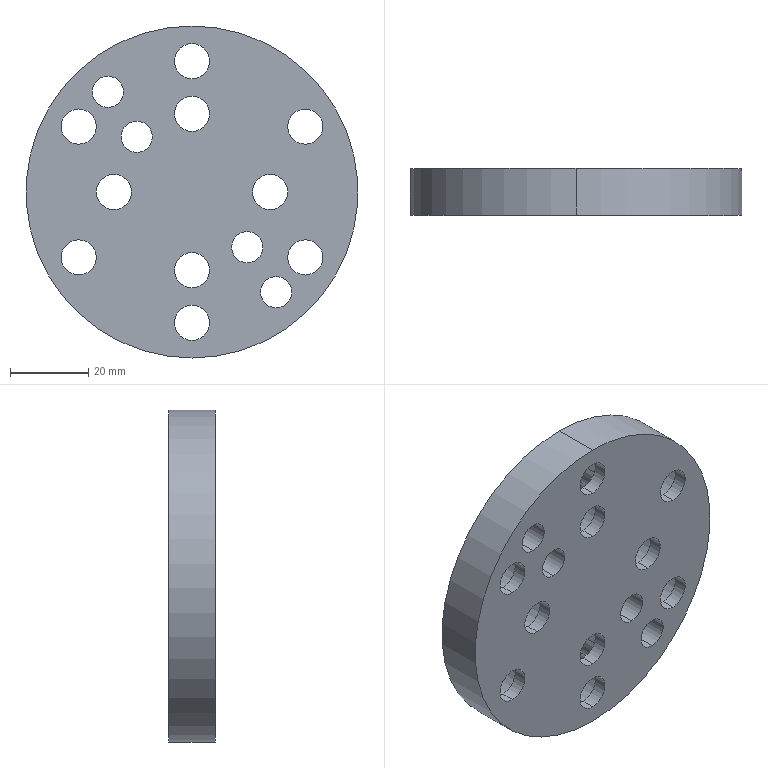Part | SolidWorks | features BaseBody 1 | 1 solid | 62 faces | box 85 x 12 x 85 mm | volume 48417 mm3 | cylinder 52 | plane 10 | commonest cylinder face diameters 9 x20 15 x18 8 x8 10 x4 85 x2